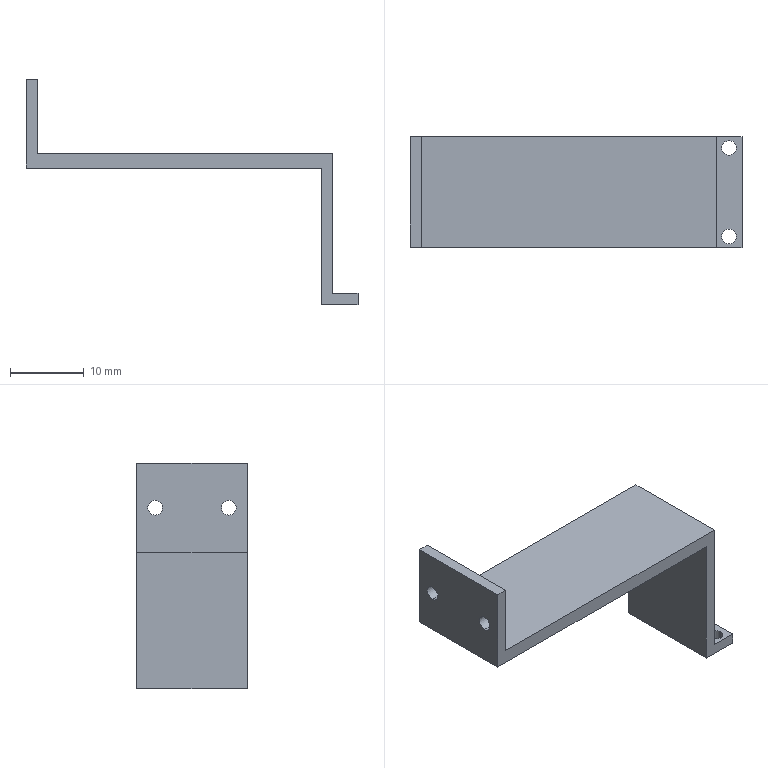Part | SolidWorks | features ICE 5, Extrusion 1 | 1 solid | 20 faces | box 45 x 15 x 30.5 mm | volume 1946 mm3 | plane 12 | cylinder 8 | commonest cylinder face diameters 2 x8
STEP:
#1=CARTESIAN_POINT('',(-41.,5.,23.5));
#2=VERTEX_POINT('',#1);
#3=CARTESIAN_POINT('',(-41.,5.,25.5));
#4=VERTEX_POINT('',#3);
#5=CARTESIAN_POINT('',(-41.,5.,24.5));
#6=DIRECTION('',(-1.,0.,0.));
#7=DIRECTION('',(0.,0.,1.));
#8=AXIS2_PLACEMENT_3D('',#5,#6,#7);
#9=CIRCLE('',#8,1.);
#10=EDGE_CURVE('',#2,#4,#9,.T.);
#11=ORIENTED_EDGE('',*,*,#10,.F.);
#12=CARTESIAN_POINT('',(-42.5,5.,23.5));
#13=VERTEX_POINT('',#12);
#14=CARTESIAN_POINT('',(-32.5,5.,23.5));
#15=DIRECTION('',(-1.,0.,0.));
#16=VECTOR('',#15,1000.);
#17=LINE('',#14,#16);
#18=EDGE_CURVE('',#2,#13,#17,.T.);
#19=ORIENTED_EDGE('',*,*,#18,.T.);
#20=CARTESIAN_POINT('',(-42.5,5.,25.5));
#21=VERTEX_POINT('',#20);
#22=CARTESIAN_POINT('',(-42.5,5.,24.5));
#23=DIRECTION('',(-1.,0.,0.));
#24=DIRECTION('',(0.,0.,1.));
#25=AXIS2_PLACEMENT_3D('',#22,#23,#24);
#26=CIRCLE('',#25,1.);
#27=EDGE_CURVE('',#13,#21,#26,.T.);
#28=ORIENTED_EDGE('',*,*,#27,.T.);
#29=CARTESIAN_POINT('',(-32.5,5.,25.5));
#30=DIRECTION('',(-1.,0.,0.));
#31=VECTOR('',#30,1000.);
#32=LINE('',#29,#31);
#33=EDGE_CURVE('',#4,#21,#32,.T.);
#34=ORIENTED_EDGE('',*,*,#33,.F.);
#35=EDGE_LOOP('',(#11,#19,#28,#34));
#36=FACE_OUTER_BOUND('',#35,.T.);
#37=CARTESIAN_POINT('',(-32.5,5.,24.5));
#38=DIRECTION('',(-1.,0.,0.));
#39=DIRECTION('',(0.,0.,1.));
#40=AXIS2_PLACEMENT_3D('',#37,#38,#39);
#41=CYLINDRICAL_SURFACE('',#40,1.);
#42=ADVANCED_FACE('',(#36),#41,.F.);
#43=CARTESIAN_POINT('',(-41.,-5.,23.5));
#44=VERTEX_POINT('',#43);
#45=CARTESIAN_POINT('',(-41.,-5.,25.5));
#46=VERTEX_POINT('',#45);
#47=CARTESIAN_POINT('',(-41.,-5.,24.5));
#48=DIRECTION('',(-1.,0.,0.));
#49=DIRECTION('',(0.,0.,1.));
#50=AXIS2_PLACEMENT_3D('',#47,#48,#49);
#51=CIRCLE('',#50,1.);
#52=EDGE_CURVE('',#44,#46,#51,.T.);
#53=ORIENTED_EDGE('',*,*,#52,.F.);
#54=CARTESIAN_POINT('',(-42.5,-5.,23.5));
#55=VERTEX_POINT('',#54);
#56=CARTESIAN_POINT('',(-32.5,-5.,23.5));
#57=DIRECTION('',(-1.,0.,0.));
#58=VECTOR('',#57,1000.);
#59=LINE('',#56,#58);
#60=EDGE_CURVE('',#44,#55,#59,.T.);
#61=ORIENTED_EDGE('',*,*,#60,.T.);
#62=CARTESIAN_POINT('',(-42.5,-5.,25.5));
#63=VERTEX_POINT('',#62);
#64=CARTESIAN_POINT('',(-42.5,-5.,24.5));
#65=DIRECTION('',(-1.,0.,0.));
#66=DIRECTION('',(0.,0.,-1.));
#67=AXIS2_PLACEMENT_3D('',#64,#65,#66);
#68=CIRCLE('',#67,1.);
#69=EDGE_CURVE('',#55,#63,#68,.T.);
#70=ORIENTED_EDGE('',*,*,#69,.T.);
#71=CARTESIAN_POINT('',(-32.5,-5.,25.5));
#72=DIRECTION('',(-1.,0.,0.));
#73=VECTOR('',#72,1000.);
#74=LINE('',#71,#73);
#75=EDGE_CURVE('',#46,#63,#74,.T.);
#76=ORIENTED_EDGE('',*,*,#75,.F.);
#77=EDGE_LOOP('',(#53,#61,#70,#76));
#78=FACE_OUTER_BOUND('',#77,.T.);
#79=CARTESIAN_POINT('',(-32.5,-5.,24.5));
#80=DIRECTION('',(-1.,0.,0.));
#81=DIRECTION('',(0.,0.,1.));
#82=AXIS2_PLACEMENT_3D('',#79,#80,#81);
#83=CYLINDRICAL_SURFACE('',#82,1.);
#84=ADVANCED_FACE('',(#78),#83,.F.);
#85=CARTESIAN_POINT('',(-0.25,6.,0.));
#86=VERTEX_POINT('',#85);
#87=CARTESIAN_POINT('',(1.75,6.,0.));
#88=VERTEX_POINT('',#87);
#89=CARTESIAN_POINT('',(0.75,6.,0.));
#90=DIRECTION('',(0.,0.,1.));
#91=DIRECTION('',(1.,0.,0.));
#92=AXIS2_PLACEMENT_3D('',#89,#90,#91);
#93=CIRCLE('',#92,1.);
#94=EDGE_CURVE('',#86,#88,#93,.T.);
#95=ORIENTED_EDGE('',*,*,#94,.F.);
#96=CARTESIAN_POINT('',(-0.25,6.,1.5));
#97=VERTEX_POINT('',#96);
#98=CARTESIAN_POINT('',(-0.25,6.,0.));
#99=DIRECTION('',(0.,0.,1.));
#100=VECTOR('',#99,1000.);
#101=LINE('',#98,#100);
#102=EDGE_CURVE('',#86,#97,#101,.T.);
#103=ORIENTED_EDGE('',*,*,#102,.T.);
#104=CARTESIAN_POINT('',(1.75,6.,1.5));
#105=VERTEX_POINT('',#104);
#106=CARTESIAN_POINT('',(0.75,6.,1.5));
#107=DIRECTION('',(0.,0.,1.));
#108=DIRECTION('',(1.,0.,0.));
#109=AXIS2_PLACEMENT_3D('',#106,#107,#108);
#110=CIRCLE('',#109,1.);
#111=EDGE_CURVE('',#97,#105,#110,.T.);
#112=ORIENTED_EDGE('',*,*,#111,.T.);
#113=CARTESIAN_POINT('',(1.75,6.,0.));
#114=DIRECTION('',(0.,0.,1.));
#115=VECTOR('',#114,1000.);
#116=LINE('',#113,#115);
#117=EDGE_CURVE('',#88,#105,#116,.T.);
#118=ORIENTED_EDGE('',*,*,#117,.F.);
#119=EDGE_LOOP('',(#95,#103,#112,#118));
#120=FACE_OUTER_BOUND('',#119,.T.);
#121=CARTESIAN_POINT('',(0.75,6.,0.));
#122=DIRECTION('',(0.,0.,1.));
#123=DIRECTION('',(1.,0.,0.));
#124=AXIS2_PLACEMENT_3D('',#121,#122,#123);
#125=CYLINDRICAL_SURFACE('',#124,1.);
#126=ADVANCED_FACE('',(#120),#125,.F.);
#127=CARTESIAN_POINT('',(-0.25,-6.,0.));
#128=VERTEX_POINT('',#127);
#129=CARTESIAN_POINT('',(1.75,-6.,0.));
#130=VERTEX_POINT('',#129);
#131=CARTESIAN_POINT('',(0.75,-6.,0.));
#132=DIRECTION('',(0.,0.,1.));
#133=DIRECTION('',(1.,0.,0.));
#134=AXIS2_PLACEMENT_3D('',#131,#132,#133);
#135=CIRCLE('',#134,1.);
#136=EDGE_CURVE('',#128,#130,#135,.T.);
#137=ORIENTED_EDGE('',*,*,#136,.F.);
#138=CARTESIAN_POINT('',(-0.25,-6.,1.5));
#139=VERTEX_POINT('',#138);
#140=CARTESIAN_POINT('',(-0.25,-6.,0.));
#141=DIRECTION('',(0.,0.,1.));
#142=VECTOR('',#141,1000.);
#143=LINE('',#140,#142);
#144=EDGE_CURVE('',#128,#139,#143,.T.);
#145=ORIENTED_EDGE('',*,*,#144,.T.);
#146=CARTESIAN_POINT('',(1.75,-6.,1.5));
#147=VERTEX_POINT('',#146);
#148=CARTESIAN_POINT('',(0.75,-6.,1.5));
#149=DIRECTION('',(0.,0.,1.));
#150=DIRECTION('',(1.,0.,0.));
#151=AXIS2_PLACEMENT_3D('',#148,#149,#150);
#152=CIRCLE('',#151,1.);
#153=EDGE_CURVE('',#139,#147,#152,.T.);
#154=ORIENTED_EDGE('',*,*,#153,.T.);
#155=CARTESIAN_POINT('',(1.75,-6.,0.));
#156=DIRECTION('',(0.,0.,1.));
#157=VECTOR('',#156,1000.);
#158=LINE('',#155,#157);
#159=EDGE_CURVE('',#130,#147,#158,.T.);
#160=ORIENTED_EDGE('',*,*,#159,.F.);
#161=EDGE_LOOP('',(#137,#145,#154,#160));
#162=FACE_OUTER_BOUND('',#161,.T.);
#163=CARTESIAN_POINT('',(0.75,-6.,0.));
#164=DIRECTION('',(0.,0.,1.));
#165=DIRECTION('',(1.,0.,0.));
#166=AXIS2_PLACEMENT_3D('',#163,#164,#165);
#167=CYLINDRICAL_SURFACE('',#166,1.);
#168=ADVANCED_FACE('',(#162),#167,.F.);
#169=CARTESIAN_POINT('',(-2.5,7.5,0.));
#170=VERTEX_POINT('',#169);
#171=CARTESIAN_POINT('',(2.5,7.5,0.));
#172=VERTEX_POINT('',#171);
#173=CARTESIAN_POINT('',(0.,7.5,0.));
#174=DIRECTION('',(1.,0.,0.));
#175=VECTOR('',#174,1000.);
#176=LINE('',#173,#175);
#177=EDGE_CURVE('',#170,#172,#176,.T.);
#178=ORIENTED_EDGE('',*,*,#177,.F.);
#179=CARTESIAN_POINT('',(-2.5,7.5,18.5));
#180=VERTEX_POINT('',#179);
#181=CARTESIAN_POINT('',(-2.5,7.5,20.5));
#182=DIRECTION('',(0.,0.,-1.));
#183=VECTOR('',#182,1000.);
#184=LINE('',#181,#183);
#185=EDGE_CURVE('',#180,#170,#184,.T.);
#186=ORIENTED_EDGE('',*,*,#185,.F.);
#187=CARTESIAN_POINT('',(-42.5,7.5,18.5));
#188=VERTEX_POINT('',#187);
#189=CARTESIAN_POINT('',(-42.5,7.5,18.5));
#190=DIRECTION('',(1.,0.,0.));
#191=VECTOR('',#190,1000.);
#192=LINE('',#189,#191);
#193=EDGE_CURVE('',#188,#180,#192,.T.);
#194=ORIENTED_EDGE('',*,*,#193,.F.);
#195=CARTESIAN_POINT('',(-42.5,7.5,30.5));
#196=VERTEX_POINT('',#195);
#197=CARTESIAN_POINT('',(-42.5,7.5,20.5));
#198=DIRECTION('',(0.,0.,-1.));
#199=VECTOR('',#198,1000.);
#200=LINE('',#197,#199);
#201=EDGE_CURVE('',#196,#188,#200,.T.);
#202=ORIENTED_EDGE('',*,*,#201,.F.);
#203=CARTESIAN_POINT('',(-41.,7.5,30.5));
#204=VERTEX_POINT('',#203);
#205=CARTESIAN_POINT('',(-42.5,7.5,30.5));
#206=DIRECTION('',(-1.,0.,0.));
#207=VECTOR('',#206,1000.);
#208=LINE('',#205,#207);
#209=EDGE_CURVE('',#204,#196,#208,.T.);
#210=ORIENTED_EDGE('',*,*,#209,.F.);
#211=CARTESIAN_POINT('',(-41.,7.5,20.5));
#212=VERTEX_POINT('',#211);
#213=CARTESIAN_POINT('',(-41.,7.5,30.5));
#214=DIRECTION('',(0.,0.,-1.));
#215=VECTOR('',#214,1000.);
#216=LINE('',#213,#215);
#217=EDGE_CURVE('',#204,#212,#216,.T.);
#218=ORIENTED_EDGE('',*,*,#217,.T.);
#219=CARTESIAN_POINT('',(-1.,7.5,20.5));
#220=VERTEX_POINT('',#219);
#221=CARTESIAN_POINT('',(0.,7.5,20.5));
#222=DIRECTION('',(1.,0.,0.));
#223=VECTOR('',#222,1000.);
#224=LINE('',#221,#223);
#225=EDGE_CURVE('',#212,#220,#224,.T.);
#226=ORIENTED_EDGE('',*,*,#225,.T.);
#227=CARTESIAN_POINT('',(-1.,7.5,1.5));
#228=VERTEX_POINT('',#227);
#229=CARTESIAN_POINT('',(-1.,7.5,20.5));
#230=DIRECTION('',(0.,0.,-1.));
#231=VECTOR('',#230,1000.);
#232=LINE('',#229,#231);
#233=EDGE_CURVE('',#220,#228,#232,.T.);
#234=ORIENTED_EDGE('',*,*,#233,.T.);
#235=CARTESIAN_POINT('',(2.5,7.5,1.5));
#236=VERTEX_POINT('',#235);
#237=CARTESIAN_POINT('',(0.,7.5,1.5));
#238=DIRECTION('',(1.,0.,0.));
#239=VECTOR('',#238,1000.);
#240=LINE('',#237,#239);
#241=EDGE_CURVE('',#228,#236,#240,.T.);
#242=ORIENTED_EDGE('',*,*,#241,.T.);
#243=CARTESIAN_POINT('',(2.5,7.5,1.5));
#244=DIRECTION('',(0.,0.,-1.));
#245=VECTOR('',#244,1000.);
#246=LINE('',#243,#245);
#247=EDGE_CURVE('',#236,#172,#246,.T.);
#248=ORIENTED_EDGE('',*,*,#247,.T.);
#249=EDGE_LOOP('',(#178,#186,#194,#202,#210,#218,#226,#234,#242,#248));
#250=FACE_OUTER_BOUND('',#249,.T.);
#251=CARTESIAN_POINT('',(0.,7.5,20.5));
#252=DIRECTION('',(0.,1.,0.));
#253=DIRECTION('',(0.,0.,1.));
#254=AXIS2_PLACEMENT_3D('',#251,#252,#253);
#255=PLANE('',#254);
#256=ADVANCED_FACE('',(#250),#255,.T.);
#257=CARTESIAN_POINT('',(-2.5,-7.5,18.5));
#258=VERTEX_POINT('',#257);
#259=CARTESIAN_POINT('',(-2.5,7.5,18.5));
#260=DIRECTION('',(0.,-1.,0.));
#261=VECTOR('',#260,1000.);
#262=LINE('',#259,#261);
#263=EDGE_CURVE('',#180,#258,#262,.T.);
#264=ORIENTED_EDGE('',*,*,#263,.F.);
#265=ORIENTED_EDGE('',*,*,#185,.T.);
#266=CARTESIAN_POINT('',(-2.5,-7.5,0.));
#267=VERTEX_POINT('',#266);
#268=CARTESIAN_POINT('',(-2.5,0.,0.));
#269=DIRECTION('',(0.,1.,0.));
#270=VECTOR('',#269,1000.);
#271=LINE('',#268,#270);
#272=EDGE_CURVE('',#267,#170,#271,.T.);
#273=ORIENTED_EDGE('',*,*,#272,.F.);
#274=CARTESIAN_POINT('',(-2.5,-7.5,20.5));
#275=DIRECTION('',(0.,0.,-1.));
#276=VECTOR('',#275,1000.);
#277=LINE('',#274,#276);
#278=EDGE_CURVE('',#258,#267,#277,.T.);
#279=ORIENTED_EDGE('',*,*,#278,.F.);
#280=EDGE_LOOP('',(#264,#265,#273,#279));
#281=FACE_OUTER_BOUND('',#280,.T.);
#282=CARTESIAN_POINT('',(-2.5,0.,20.5));
#283=DIRECTION('',(-1.,0.,0.));
#284=DIRECTION('',(0.,0.,1.));
#285=AXIS2_PLACEMENT_3D('',#282,#283,#284);
#286=PLANE('',#285);
#287=ADVANCED_FACE('',(#281),#286,.T.);
#288=CARTESIAN_POINT('',(2.5,-7.5,0.));
#289=VERTEX_POINT('',#288);
#290=CARTESIAN_POINT('',(0.,-7.5,0.));
#291=DIRECTION('',(1.,0.,0.));
#292=VECTOR('',#291,1000.);
#293=LINE('',#290,#292);
#294=EDGE_CURVE('',#267,#289,#293,.T.);
#295=ORIENTED_EDGE('',*,*,#294,.T.);
#296=CARTESIAN_POINT('',(2.5,-7.5,1.5));
#297=VERTEX_POINT('',#296);
#298=CARTESIAN_POINT('',(2.5,-7.5,1.5));
#299=DIRECTION('',(0.,0.,-1.));
#300=VECTOR('',#299,1000.);
#301=LINE('',#298,#300);
#302=EDGE_CURVE('',#297,#289,#301,.T.);
#303=ORIENTED_EDGE('',*,*,#302,.F.);
#304=CARTESIAN_POINT('',(-1.,-7.5,1.5));
#305=VERTEX_POINT('',#304);
#306=CARTESIAN_POINT('',(0.,-7.5,1.5));
#307=DIRECTION('',(1.,0.,0.));
#308=VECTOR('',#307,1000.);
#309=LINE('',#306,#308);
#310=EDGE_CURVE('',#305,#297,#309,.T.);
#311=ORIENTED_EDGE('',*,*,#310,.F.);
#312=CARTESIAN_POINT('',(-1.,-7.5,20.5));
#313=VERTEX_POINT('',#312);
#314=CARTESIAN_POINT('',(-1.,-7.5,20.5));
#315=DIRECTION('',(0.,0.,-1.));
#316=VECTOR('',#315,1000.);
#317=LINE('',#314,#316);
#318=EDGE_CURVE('',#313,#305,#317,.T.);
#319=ORIENTED_EDGE('',*,*,#318,.F.);
#320=CARTESIAN_POINT('',(-41.,-7.5,20.5));
#321=VERTEX_POINT('',#320);
#322=CARTESIAN_POINT('',(0.,-7.5,20.5));
#323=DIRECTION('',(1.,0.,0.));
#324=VECTOR('',#323,1000.);
#325=LINE('',#322,#324);
#326=EDGE_CURVE('',#321,#313,#325,.T.);
#327=ORIENTED_EDGE('',*,*,#326,.F.);
#328=CARTESIAN_POINT('',(-41.,-7.5,30.5));
#329=VERTEX_POINT('',#328);
#330=CARTESIAN_POINT('',(-41.,-7.5,30.5));
#331=DIRECTION('',(0.,0.,-1.));
#332=VECTOR('',#331,1000.);
#333=LINE('',#330,#332);
#334=EDGE_CURVE('',#329,#321,#333,.T.);
#335=ORIENTED_EDGE('',*,*,#334,.F.);
#336=CARTESIAN_POINT('',(-42.5,-7.5,30.5));
#337=VERTEX_POINT('',#336);
#338=CARTESIAN_POINT('',(-42.5,-7.5,30.5));
#339=DIRECTION('',(1.,0.,0.));
#340=VECTOR('',#339,1000.);
#341=LINE('',#338,#340);
#342=EDGE_CURVE('',#337,#329,#341,.T.);
#343=ORIENTED_EDGE('',*,*,#342,.F.);
#344=CARTESIAN_POINT('',(-42.5,-7.5,18.5));
#345=VERTEX_POINT('',#344);
#346=CARTESIAN_POINT('',(-42.5,-7.5,20.5));
#347=DIRECTION('',(0.,0.,1.));
#348=VECTOR('',#347,1000.);
#349=LINE('',#346,#348);
#350=EDGE_CURVE('',#345,#337,#349,.T.);
#351=ORIENTED_EDGE('',*,*,#350,.F.);
#352=CARTESIAN_POINT('',(-42.5,-7.5,18.5));
#353=DIRECTION('',(1.,0.,0.));
#354=VECTOR('',#353,1000.);
#355=LINE('',#352,#354);
#356=EDGE_CURVE('',#345,#258,#355,.T.);
#357=ORIENTED_EDGE('',*,*,#356,.T.);
#358=ORIENTED_EDGE('',*,*,#278,.T.);
#359=EDGE_LOOP('',(#295,#303,#311,#319,#327,#335,#343,#351,#357,#358));
#360=FACE_OUTER_BOUND('',#359,.T.);
#361=CARTESIAN_POINT('',(0.,-7.5,20.5));
#362=DIRECTION('',(0.,1.,0.));
#363=DIRECTION('',(0.,0.,1.));
#364=AXIS2_PLACEMENT_3D('',#361,#362,#363);
#365=PLANE('',#364);
#366=ADVANCED_FACE('',(#360),#365,.F.);
#367=CARTESIAN_POINT('',(-1.,0.,1.5));
#368=DIRECTION('',(0.,-1.,0.));
#369=VECTOR('',#368,1000.);
#370=LINE('',#367,#369);
#371=EDGE_CURVE('',#228,#305,#370,.T.);
#372=ORIENTED_EDGE('',*,*,#371,.F.);
#373=ORIENTED_EDGE('',*,*,#233,.F.);
#374=CARTESIAN_POINT('',(-1.,0.,20.5));
#375=DIRECTION('',(0.,-1.,0.));
#376=VECTOR('',#375,1000.);
#377=LINE('',#374,#376);
#378=EDGE_CURVE('',#220,#313,#377,.T.);
#379=ORIENTED_EDGE('',*,*,#378,.T.);
#380=ORIENTED_EDGE('',*,*,#318,.T.);
#381=EDGE_LOOP('',(#372,#373,#379,#380));
#382=FACE_OUTER_BOUND('',#381,.T.);
#383=CARTESIAN_POINT('',(-1.,0.,20.5));
#384=DIRECTION('',(1.,0.,0.));
#385=DIRECTION('',(0.,1.,0.));
#386=AXIS2_PLACEMENT_3D('',#383,#384,#385);
#387=PLANE('',#386);
#388=ADVANCED_FACE('',(#382),#387,.T.);
#389=CARTESIAN_POINT('',(-41.,7.5,20.5));
#390=DIRECTION('',(0.,1.,0.));
#391=VECTOR('',#390,1000.);
#392=LINE('',#389,#391);
#393=EDGE_CURVE('',#321,#212,#392,.T.);
#394=ORIENTED_EDGE('',*,*,#393,.F.);
#395=ORIENTED_EDGE('',*,*,#326,.T.);
#396=ORIENTED_EDGE('',*,*,#378,.F.);
#397=ORIENTED_EDGE('',*,*,#225,.F.);
#398=EDGE_LOOP('',(#394,#395,#396,#397));
#399=FACE_OUTER_BOUND('',#398,.T.);
#400=CARTESIAN_POINT('',(0.,0.,20.5));
#401=DIRECTION('',(0.,0.,1.));
#402=DIRECTION('',(1.,0.,0.));
#403=AXIS2_PLACEMENT_3D('',#400,#401,#402);
#404=PLANE('',#403);
#405=ADVANCED_FACE('',(#399),#404,.T.);
#406=CARTESIAN_POINT('',(0.75,6.,0.));
#407=DIRECTION('',(0.,0.,1.));
#408=DIRECTION('',(1.,0.,0.));
#409=AXIS2_PLACEMENT_3D('',#406,#407,#408);
#410=CIRCLE('',#409,1.);
#411=EDGE_CURVE('',#88,#86,#410,.T.);
#412=ORIENTED_EDGE('',*,*,#411,.T.);
#413=ORIENTED_EDGE('',*,*,#94,.T.);
#414=EDGE_LOOP('',(#412,#413));
#415=FACE_BOUND('',#414,.T.);
#416=CARTESIAN_POINT('',(0.75,-6.,0.));
#417=DIRECTION('',(0.,0.,1.));
#418=DIRECTION('',(1.,0.,0.));
#419=AXIS2_PLACEMENT_3D('',#416,#417,#418);
#420=CIRCLE('',#419,1.);
#421=EDGE_CURVE('',#130,#128,#420,.T.);
#422=ORIENTED_EDGE('',*,*,#421,.T.);
#423=ORIENTED_EDGE('',*,*,#136,.T.);
#424=EDGE_LOOP('',(#422,#423));
#425=FACE_BOUND('',#424,.T.);
#426=ORIENTED_EDGE('',*,*,#177,.T.);
#427=CARTESIAN_POINT('',(2.5,0.,0.));
#428=DIRECTION('',(0.,1.,0.));
#429=VECTOR('',#428,1000.);
#430=LINE('',#427,#429);
#431=EDGE_CURVE('',#289,#172,#430,.T.);
#432=ORIENTED_EDGE('',*,*,#431,.F.);
#433=ORIENTED_EDGE('',*,*,#294,.F.);
#434=ORIENTED_EDGE('',*,*,#272,.T.);
#435=EDGE_LOOP('',(#426,#432,#433,#434));
#436=FACE_OUTER_BOUND('',#435,.T.);
#437=CARTESIAN_POINT('',(0.,0.,0.));
#438=DIRECTION('',(0.,0.,1.));
#439=DIRECTION('',(1.,0.,0.));
#440=AXIS2_PLACEMENT_3D('',#437,#438,#439);
#441=PLANE('',#440);
#442=ADVANCED_FACE('',(#415,#425,#436),#441,.F.);
#443=ORIENTED_EDGE('',*,*,#431,.T.);
#444=ORIENTED_EDGE('',*,*,#247,.F.);
#445=CARTESIAN_POINT('',(2.5,0.,1.5));
#446=DIRECTION('',(0.,1.,0.));
#447=VECTOR('',#446,1000.);
#448=LINE('',#445,#447);
#449=EDGE_CURVE('',#297,#236,#448,.T.);
#450=ORIENTED_EDGE('',*,*,#449,.F.);
#451=ORIENTED_EDGE('',*,*,#302,.T.);
#452=EDGE_LOOP('',(#443,#444,#450,#451));
#453=FACE_OUTER_BOUND('',#452,.T.);
#454=CARTESIAN_POINT('',(2.5,0.,1.5));
#455=DIRECTION('',(-1.,0.,0.));
#456=DIRECTION('',(0.,0.,1.));
#457=AXIS2_PLACEMENT_3D('',#454,#455,#456);
#458=PLANE('',#457);
#459=ADVANCED_FACE('',(#453),#458,.F.);
#460=CARTESIAN_POINT('',(0.75,6.,1.5));
#461=DIRECTION('',(0.,0.,1.));
#462=DIRECTION('',(1.,0.,0.));
#463=AXIS2_PLACEMENT_3D('',#460,#461,#462);
#464=CIRCLE('',#463,1.);
#465=EDGE_CURVE('',#105,#97,#464,.T.);
#466=ORIENTED_EDGE('',*,*,#465,.F.);
#467=ORIENTED_EDGE('',*,*,#111,.F.);
#468=EDGE_LOOP('',(#466,#467));
#469=FACE_BOUND('',#468,.T.);
#470=CARTESIAN_POINT('',(0.75,-6.,1.5));
#471=DIRECTION('',(0.,0.,1.));
#472=DIRECTION('',(1.,0.,0.));
#473=AXIS2_PLACEMENT_3D('',#470,#471,#472);
#474=CIRCLE('',#473,1.);
#475=EDGE_CURVE('',#147,#139,#474,.T.);
#476=ORIENTED_EDGE('',*,*,#475,.F.);
#477=ORIENTED_EDGE('',*,*,#153,.F.);
#478=EDGE_LOOP('',(#476,#477));
#479=FACE_BOUND('',#478,.T.);
#480=ORIENTED_EDGE('',*,*,#310,.T.);
#481=ORIENTED_EDGE('',*,*,#449,.T.);
#482=ORIENTED_EDGE('',*,*,#241,.F.);
#483=ORIENTED_EDGE('',*,*,#371,.T.);
#484=EDGE_LOOP('',(#480,#481,#482,#483));
#485=FACE_OUTER_BOUND('',#484,.T.);
#486=CARTESIAN_POINT('',(0.,0.,1.5));
#487=DIRECTION('',(0.,0.,1.));
#488=DIRECTION('',(1.,0.,0.));
#489=AXIS2_PLACEMENT_3D('',#486,#487,#488);
#490=PLANE('',#489);
#491=ADVANCED_FACE('',(#469,#479,#485),#490,.T.);
#492=ORIENTED_EDGE('',*,*,#144,.F.);
#493=ORIENTED_EDGE('',*,*,#421,.F.);
#494=ORIENTED_EDGE('',*,*,#159,.T.);
#495=ORIENTED_EDGE('',*,*,#475,.T.);
#496=EDGE_LOOP('',(#492,#493,#494,#495));
#497=FACE_OUTER_BOUND('',#496,.T.);
#498=CARTESIAN_POINT('',(0.75,-6.,0.));
#499=DIRECTION('',(0.,0.,1.));
#500=DIRECTION('',(1.,0.,0.));
#501=AXIS2_PLACEMENT_3D('',#498,#499,#500);
#502=CYLINDRICAL_SURFACE('',#501,1.);
#503=ADVANCED_FACE('',(#497),#502,.F.);
#504=ORIENTED_EDGE('',*,*,#102,.F.);
#505=ORIENTED_EDGE('',*,*,#411,.F.);
#506=ORIENTED_EDGE('',*,*,#117,.T.);
#507=ORIENTED_EDGE('',*,*,#465,.T.);
#508=EDGE_LOOP('',(#504,#505,#506,#507));
#509=FACE_OUTER_BOUND('',#508,.T.);
#510=CARTESIAN_POINT('',(0.75,6.,0.));
#511=DIRECTION('',(0.,0.,1.));
#512=DIRECTION('',(1.,0.,0.));
#513=AXIS2_PLACEMENT_3D('',#510,#511,#512);
#514=CYLINDRICAL_SURFACE('',#513,1.);
#515=ADVANCED_FACE('',(#509),#514,.F.);
#516=ORIENTED_EDGE('',*,*,#263,.T.);
#517=ORIENTED_EDGE('',*,*,#356,.F.);
#518=CARTESIAN_POINT('',(-42.5,7.5,18.5));
#519=DIRECTION('',(0.,-1.,0.));
#520=VECTOR('',#519,1000.);
#521=LINE('',#518,#520);
#522=EDGE_CURVE('',#188,#345,#521,.T.);
#523=ORIENTED_EDGE('',*,*,#522,.F.);
#524=ORIENTED_EDGE('',*,*,#193,.T.);
#525=EDGE_LOOP('',(#516,#517,#523,#524));
#526=FACE_OUTER_BOUND('',#525,.T.);
#527=CARTESIAN_POINT('',(-42.5,7.5,18.5));
#528=DIRECTION('',(0.,0.,1.));
#529=DIRECTION('',(1.,0.,0.));
#530=AXIS2_PLACEMENT_3D('',#527,#528,#529);
#531=PLANE('',#530);
#532=ADVANCED_FACE('',(#526),#531,.F.);
#533=CARTESIAN_POINT('',(-42.5,5.,24.5));
#534=DIRECTION('',(-1.,0.,0.));
#535=DIRECTION('',(0.,0.,1.));
#536=AXIS2_PLACEMENT_3D('',#533,#534,#535);
#537=CIRCLE('',#536,1.);
#538=EDGE_CURVE('',#21,#13,#537,.T.);
#539=ORIENTED_EDGE('',*,*,#538,.F.);
#540=ORIENTED_EDGE('',*,*,#27,.F.);
#541=EDGE_LOOP('',(#539,#540));
#542=FACE_BOUND('',#541,.T.);
#543=CARTESIAN_POINT('',(-42.5,-5.,24.5));
#544=DIRECTION('',(-1.,0.,0.));
#545=DIRECTION('',(0.,0.,-1.));
#546=AXIS2_PLACEMENT_3D('',#543,#544,#545);
#547=CIRCLE('',#546,1.);
#548=EDGE_CURVE('',#63,#55,#547,.T.);
#549=ORIENTED_EDGE('',*,*,#548,.F.);
#550=ORIENTED_EDGE('',*,*,#69,.F.);
#551=EDGE_LOOP('',(#549,#550));
#552=FACE_BOUND('',#551,.T.);
#553=ORIENTED_EDGE('',*,*,#350,.T.);
#554=CARTESIAN_POINT('',(-42.5,7.5,30.5));
#555=DIRECTION('',(0.,-1.,0.));
#556=VECTOR('',#555,1000.);
#557=LINE('',#554,#556);
#558=EDGE_CURVE('',#196,#337,#557,.T.);
#559=ORIENTED_EDGE('',*,*,#558,.F.);
#560=ORIENTED_EDGE('',*,*,#201,.T.);
#561=ORIENTED_EDGE('',*,*,#522,.T.);
#562=EDGE_LOOP('',(#553,#559,#560,#561));
#563=FACE_OUTER_BOUND('',#562,.T.);
#564=CARTESIAN_POINT('',(-42.5,0.,0.));
#565=DIRECTION('',(1.,0.,0.));
#566=DIRECTION('',(0.,0.,-1.));
#567=AXIS2_PLACEMENT_3D('',#564,#565,#566);
#568=PLANE('',#567);
#569=ADVANCED_FACE('',(#542,#552,#563),#568,.F.);
#570=CARTESIAN_POINT('',(-41.,5.,24.5));
#571=DIRECTION('',(-1.,0.,0.));
#572=DIRECTION('',(0.,0.,1.));
#573=AXIS2_PLACEMENT_3D('',#570,#571,#572);
#574=CIRCLE('',#573,1.);
#575=EDGE_CURVE('',#4,#2,#574,.T.);
#576=ORIENTED_EDGE('',*,*,#575,.T.);
#577=ORIENTED_EDGE('',*,*,#10,.T.);
#578=EDGE_LOOP('',(#576,#577));
#579=FACE_BOUND('',#578,.T.);
#580=CARTESIAN_POINT('',(-41.,-5.,24.5));
#581=DIRECTION('',(-1.,0.,0.));
#582=DIRECTION('',(0.,0.,1.));
#583=AXIS2_PLACEMENT_3D('',#580,#581,#582);
#584=CIRCLE('',#583,1.);
#585=EDGE_CURVE('',#46,#44,#584,.T.);
#586=ORIENTED_EDGE('',*,*,#585,.T.);
#587=ORIENTED_EDGE('',*,*,#52,.T.);
#588=EDGE_LOOP('',(#586,#587));
#589=FACE_BOUND('',#588,.T.);
#590=ORIENTED_EDGE('',*,*,#393,.T.);
#591=ORIENTED_EDGE('',*,*,#217,.F.);
#592=CARTESIAN_POINT('',(-41.,7.5,30.5));
#593=DIRECTION('',(0.,1.,0.));
#594=VECTOR('',#593,1000.);
#595=LINE('',#592,#594);
#596=EDGE_CURVE('',#329,#204,#595,.T.);
#597=ORIENTED_EDGE('',*,*,#596,.F.);
#598=ORIENTED_EDGE('',*,*,#334,.T.);
#599=EDGE_LOOP('',(#590,#591,#597,#598));
#600=FACE_OUTER_BOUND('',#599,.T.);
#601=CARTESIAN_POINT('',(-41.,7.5,30.5));
#602=DIRECTION('',(-1.,0.,0.));
#603=DIRECTION('',(0.,0.,1.));
#604=AXIS2_PLACEMENT_3D('',#601,#602,#603);
#605=PLANE('',#604);
#606=ADVANCED_FACE('',(#579,#589,#600),#605,.F.);
#607=ORIENTED_EDGE('',*,*,#558,.T.);
#608=ORIENTED_EDGE('',*,*,#342,.T.);
#609=ORIENTED_EDGE('',*,*,#596,.T.);
#610=ORIENTED_EDGE('',*,*,#209,.T.);
#611=EDGE_LOOP('',(#607,#608,#609,#610));
#612=FACE_OUTER_BOUND('',#611,.T.);
#613=CARTESIAN_POINT('',(0.,0.,30.5));
#614=DIRECTION('',(0.,0.,1.));
#615=DIRECTION('',(1.,0.,0.));
#616=AXIS2_PLACEMENT_3D('',#613,#614,#615);
#617=PLANE('',#616);
#618=ADVANCED_FACE('',(#612),#617,.T.);
#619=ORIENTED_EDGE('',*,*,#60,.F.);
#620=ORIENTED_EDGE('',*,*,#585,.F.);
#621=ORIENTED_EDGE('',*,*,#75,.T.);
#622=ORIENTED_EDGE('',*,*,#548,.T.);
#623=EDGE_LOOP('',(#619,#620,#621,#622));
#624=FACE_OUTER_BOUND('',#623,.T.);
#625=CARTESIAN_POINT('',(-32.5,-5.,24.5));
#626=DIRECTION('',(-1.,0.,0.));
#627=DIRECTION('',(0.,0.,1.));
#628=AXIS2_PLACEMENT_3D('',#625,#626,#627);
#629=CYLINDRICAL_SURFACE('',#628,1.);
#630=ADVANCED_FACE('',(#624),#629,.F.);
#631=ORIENTED_EDGE('',*,*,#18,.F.);
#632=ORIENTED_EDGE('',*,*,#575,.F.);
#633=ORIENTED_EDGE('',*,*,#33,.T.);
#634=ORIENTED_EDGE('',*,*,#538,.T.);
#635=EDGE_LOOP('',(#631,#632,#633,#634));
#636=FACE_OUTER_BOUND('',#635,.T.);
#637=CARTESIAN_POINT('',(-32.5,5.,24.5));
#638=DIRECTION('',(-1.,0.,0.));
#639=DIRECTION('',(0.,0.,1.));
#640=AXIS2_PLACEMENT_3D('',#637,#638,#639);
#641=CYLINDRICAL_SURFACE('',#640,1.);
#642=ADVANCED_FACE('',(#636),#641,.F.);
#643=CLOSED_SHELL('',(#42,#84,#126,#168,#256,#287,#366,#388,#405,#442,#459,#491,#503,#515,#532,#569,#606,#618,#630,#642));
#644=MANIFOLD_SOLID_BREP('',#643);
#645=CARTESIAN_POINT('',(0.,0.,0.));
#646=DIRECTION('',(0.,0.,1.));
#647=DIRECTION('',(1.,0.,0.));
#648=AXIS2_PLACEMENT_3D('',#645,#646,#647);
#649=(LENGTH_UNIT()NAMED_UNIT(*)SI_UNIT(.MILLI.,.METRE.));
#650=UNCERTAINTY_MEASURE_WITH_UNIT(LENGTH_MEASURE(0.00001),#649,'','');
#651=(NAMED_UNIT(*)PLANE_ANGLE_UNIT()SI_UNIT($,.RADIAN.));
#652=(NAMED_UNIT(*)SI_UNIT($,.STERADIAN.)SOLID_ANGLE_UNIT());
#653=(GEOMETRIC_REPRESENTATION_CONTEXT(3)GLOBAL_UNCERTAINTY_ASSIGNED_CONTEXT((#650))GLOBAL_UNIT_ASSIGNED_CONTEXT((#649,#651,#652))REPRESENTATION_CONTEXT('',''));
#654=ADVANCED_BREP_SHAPE_REPRESENTATION('',(#644,#648),#653);